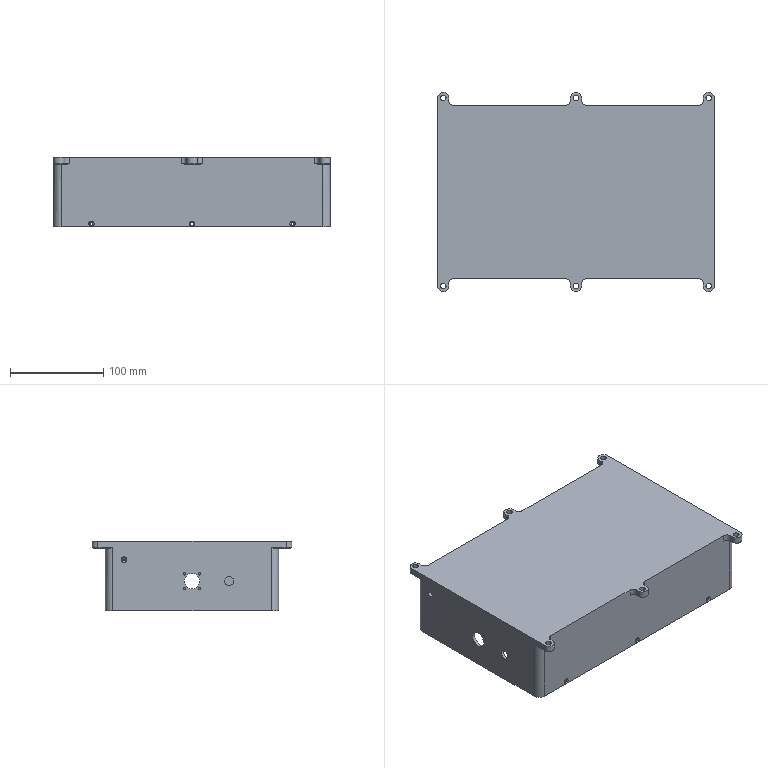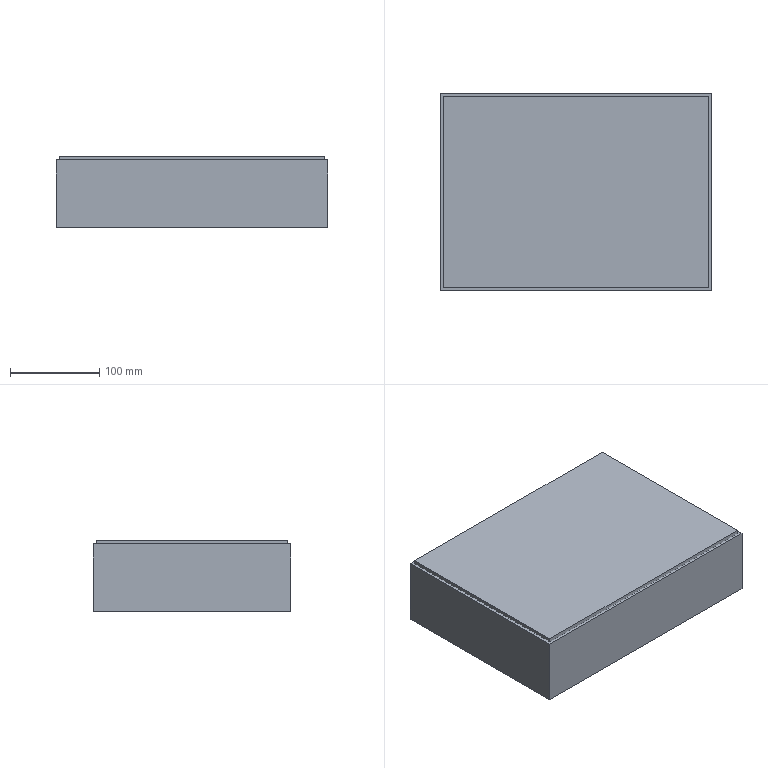CAM job | NX | 3+2 milling, drilling | part box 297 x 214 x 75 mm | stock box 304 x 221 x 80 mm
Tools:
number,name,description,diameter,corner_radius,flute_length,length,flutes
3,D63,Milling Tool-5 Parameters,63.0,0.0,50.0,75.0,2
1,D6A45,Milling Tool-5 Parameters,6.0,0.0,3.0,3.0,2
22,2.5ZT,Drilling Tool,2.5,0.0,35.0,50.0,2
20,6.0ZT,Drilling Tool,6.0,0.0,35.0,50.0,2
2,D16,Milling Tool-5 Parameters,16.0,0.0,50.0,75.0,2
14,D10JING,Milling Tool-5 Parameters,10.0,0.0,50.0,75.0,2
17,D4,Milling Tool-5 Parameters,4.0,0.0,50.0,75.0,2
4,D10,Milling Tool-5 Parameters,10.0,0.0,50.0,75.0,2
23,3.4ZT,Drilling Tool,3.4,0.0,35.0,50.0,2
12,5.5ZT,Drilling Tool,5.5,0.0,35.0,50.0,2
17,D6,Milling Tool-5 Parameters,6.0,0.0,50.0,75.0,2
20,2.1ZT,Drilling Tool,2.05,0.0,35.0,50.0,2
Operations:
program,operation,operation_type,tool,method,geometry_group,spindle_rpm,surface_speed,feed_per_tooth,feed_cut,feed_plunge,cut_length_mm,path_length_mm,cut_time_min,machine_time_min
1,FLOOR_WALL,VolumeBased25DMillingOperation,D63,METHOD,A,6500.0,1286.0,0.0962,1250.0,100.0,2042.797,2096.797,1.634,1.64
1,DRILLING_COPY_1_1,Operation,D6A45,METHOD,A,5000.0,94.0,0.025,250.0,0.0,27.3,901.749,0.1092,0.1966
1,DRILLING_COPY_COPY_1,Operation,6.0ZT,METHOD,A,2000.0,37.0,0.05,200.0,0.0,85.816,1018.78,0.4291,0.5224
1,ZLEVEL_PROFILE_COPY,ZLevelMilling,D16,METHOD,MCS_MILL,7000.0,351.0,0.1429,2000.0,1000.0,54049.523,54901.811,27.381,27.466
1,ZLEVEL_PROFILE,ZLevelMilling,D16,METHOD,A,7000.0,351.0,0.1429,2000.0,1000.0,84581.771,84713.771,42.315,42.328
1,ZLEVEL_PROFILE_1,ZLevelMilling,D16,METHOD,A,7500.0,376.0,0.0667,1000.0,100.0,5702.749,5910.556,5.703,5.723
1,CAVITY_MILL,CavityMilling,D10JING,METHOD,A,9500.0,119.0,0.0842,1600.0,100.0,939.214,2514.64,0.587,0.7446
1,ZLEVEL_PROFILE_2_COPY,ZLevelMilling,D6A45,METHOD,A,9500.0,179.0,0.0658,1250.0,100.0,1212.497,2855.118,0.97,1.134
TOPFACESETUP2,DRILLING_COPY_1_1_1,Operation,D6A45,METHOD,B,5000.0,94.0,0.025,250.0,0.0,18.0,346.083,0.072,0.1048
TOPFACESETUP2,DRILLING_COPY_COPY_1_1,Operation,3.4ZT,METHOD,B,1447.0,10.0,0.0346,100.0,0.0,25.564,361.212,0.2556,0.2892
3,ZLEVEL_PROFILE_COPY_1,ZLevelMilling,D10,METHOD,C,11173.0,351.0,0.0895,2000.0,1000.0,162.695,222.695,0.1052,0.1112
3,PLANAR_MILL_COPY_COPY_COPY_COPY_COPY,PlanarMilling,D6A45,METHOD,C,9500.0,179.0,0.0658,1250.0,100.0,61.383,121.383,0.0491,0.0551
3,TOOLCOMP17,ZLevelMilling,D4,METHOD,C,9500.0,298.0,0.0526,1000.0,100.0,54.88,118.88,0.0549,0.0613
4,DRILLING_COPY_1_1_1_COPY,Operation,D6A45,METHOD,D,5000.0,94.0,0.025,250.0,0.0,31.85,297.564,0.1274,0.154
4,DRILLING_COPY_COPY_COPY,Operation,2.5ZT,METHOD,D,1447.0,10.0,0.0346,100.0,0.0,33.004,183.845,0.33,0.3451
4,DRILLING_COPY_COPY_COPY_COPY,Operation,5.5ZT,METHOD,D,1447.0,10.0,0.0346,100.0,0.0,14.652,89.305,0.1465,0.154
4,HOLE_MILLING,CylinderMilling,D6,METHOD,D,9500.0,179.0,0.0947,1800.0,100.0,514.197,682.697,0.2857,0.3025
4,HOLE_MILLING_COPY,CylinderMilling,D6,METHOD,D,9500.0,179.0,0.0526,1000.0,100.0,146.567,311.567,0.1466,0.1631
4,PLANAR_MILL_COPY_COPY_COPY_COPY_COPY_COPY,PlanarMilling,D6A45,METHOD,D,9500.0,179.0,0.0658,1250.0,100.0,99.175,390.328,0.0793,0.1085
5,FLOOR_WALL_COPY,VolumeBased25DMillingOperation,D63,METHOD,E,6500.0,1286.0,0.0962,1250.0,100.0,10003.985,11900.388,8.003,8.193
5,FLOOR_WALL_COPY_1,VolumeBased25DMillingOperation,D63,METHOD,E,6500.0,1286.0,0.0962,1250.0,100.0,2000.797,2054.797,1.601,1.606
5,FLOOR_WALL_1,VolumeBased25DMillingOperation,D16,METHOD,E,7500.0,376.0,0.1467,2200.0,1000.0,39109.156,42820.219,19.014,19.385
5,FLOOR_WALL_1_COPY,VolumeBased25DMillingOperation,D16,METHOD,E,7500.0,376.0,0.0667,1000.0,1000.0,1081.948,5230.082,1.082,1.497
5,FLOOR_WALL_1_COPY_COPY,VolumeBased25DMillingOperation,D16,METHOD,E,7500.0,376.0,0.0667,1000.0,1000.0,270.487,2019.363,0.2705,0.4454
5,CAVITY_MILL_1,CavityMilling,D16,METHOD,E,7500.0,376.0,0.1333,2000.0,1000.0,377308.862,383831.717,190.373,191.025
5,CAVITY_MILL_COPY,CavityMilling,D10JING,METHOD,E,7500.0,235.0,0.1067,1600.0,100.0,8600.207,13381.317,5.375,5.853
5,ZLEVEL_PROFILE_1_COPY,ZLevelMilling,D10JING,METHOD,E,7500.0,376.0,0.0667,1000.0,100.0,2743.891,2897.717,2.744,2.759
5,ZLEVEL_PROFILE_1_COPY_COPY,ZLevelMilling,D10JING,METHOD,E,7500.0,376.0,0.0667,1000.0,100.0,2180.251,4740.496,2.18,2.436
5,FLOOR_WALL_1_COPY_1_COPY,VolumeBased25DMillingOperation,D10JING,METHOD,E,7500.0,235.0,0.0667,1000.0,1000.0,10145.579,15788.461,10.146,10.721
5,DRILLING_COPY_1,Operation,D6A45,METHOD,E,5000.0,94.0,0.025,250.0,0.0,24.6,865.186,0.0984,0.1825
5,DRILLING_COPY_COPY,Operation,2.1ZT,METHOD,E,1447.0,10.0,0.0346,100.0,0.0,58.595,933.176,0.586,0.6734
5,ZLEVEL_PROFILE_2_COPY_1,ZLevelMilling,D6A45,METHOD,E,9500.0,179.0,0.0658,1250.0,100.0,1898.595,2297.66,1.519,1.559